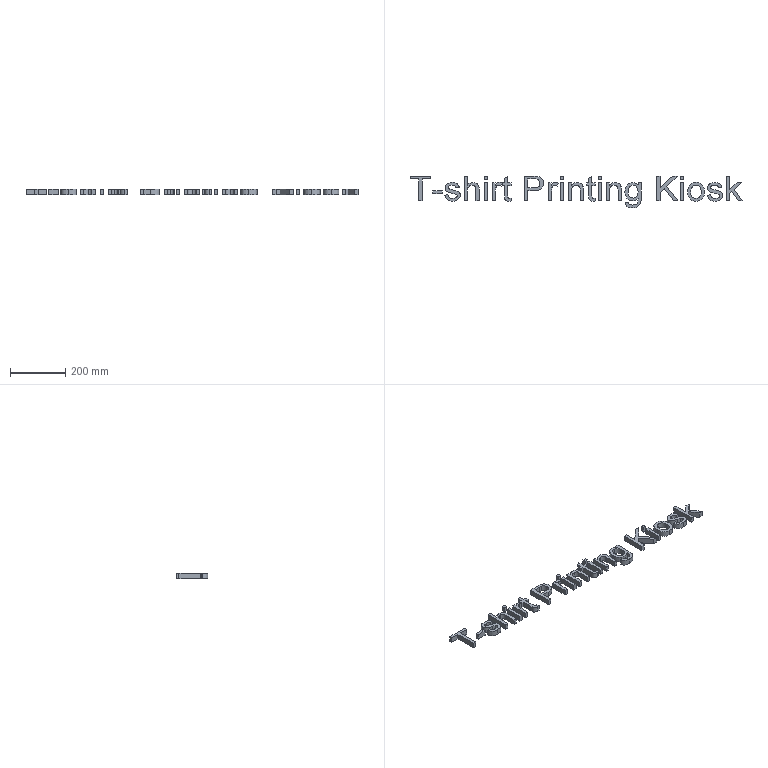Part | SolidWorks | features BaseBody 24 | 24 solids | 285 faces | box 1198 x 114.943 x 20 mm | volume 636251 mm3 | plane 192 | spline 93